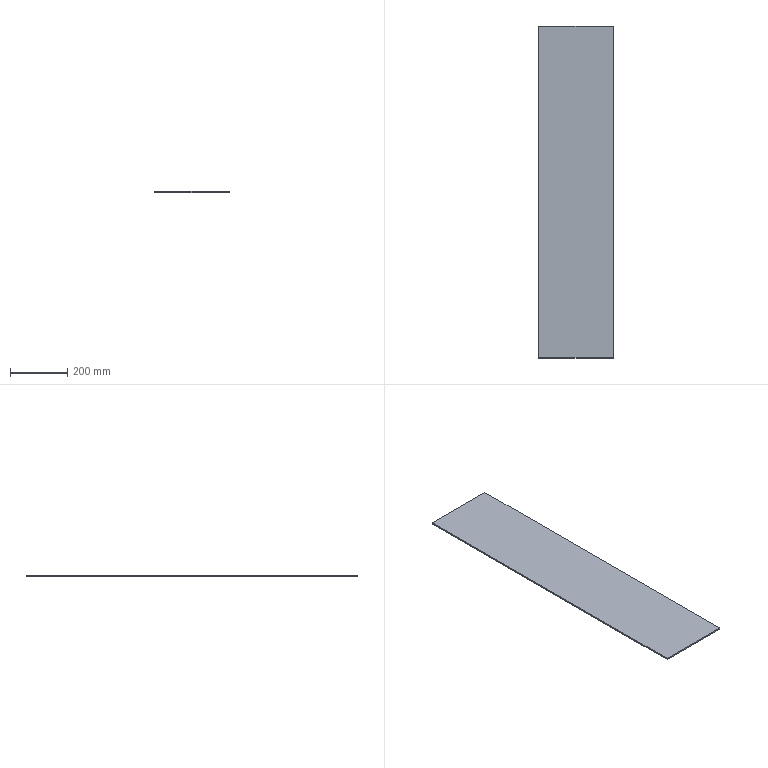Part | SolidWorks | features BaseBody 1 | 1 solid | 6 faces | box 260 x 1160 x 5 mm | volume 1508000 mm3 | plane 6
STEP:
#1=CARTESIAN_POINT('',(-860.,1800.,-395.));
#2=VERTEX_POINT('',#1);
#3=CARTESIAN_POINT('',(-600.,1800.,-395.));
#4=VERTEX_POINT('',#3);
#5=CARTESIAN_POINT('',(-860.,1800.,-395.));
#6=DIRECTION('',(1.,0.,0.));
#7=VECTOR('',#6,1000.);
#8=LINE('',#5,#7);
#9=EDGE_CURVE('',#2,#4,#8,.T.);
#10=ORIENTED_EDGE('',*,*,#9,.F.);
#11=CARTESIAN_POINT('',(-860.,640.,-395.));
#12=VERTEX_POINT('',#11);
#13=CARTESIAN_POINT('',(-860.,640.,-395.));
#14=DIRECTION('',(0.,1.,0.));
#15=VECTOR('',#14,1000.);
#16=LINE('',#13,#15);
#17=EDGE_CURVE('',#12,#2,#16,.T.);
#18=ORIENTED_EDGE('',*,*,#17,.F.);
#19=CARTESIAN_POINT('',(-600.,640.,-395.));
#20=VERTEX_POINT('',#19);
#21=CARTESIAN_POINT('',(-600.,640.,-395.));
#22=DIRECTION('',(-1.,0.,0.));
#23=VECTOR('',#22,1000.);
#24=LINE('',#21,#23);
#25=EDGE_CURVE('',#20,#12,#24,.T.);
#26=ORIENTED_EDGE('',*,*,#25,.F.);
#27=CARTESIAN_POINT('',(-600.,1800.,-395.));
#28=DIRECTION('',(0.,-1.,0.));
#29=VECTOR('',#28,1000.);
#30=LINE('',#27,#29);
#31=EDGE_CURVE('',#4,#20,#30,.T.);
#32=ORIENTED_EDGE('',*,*,#31,.F.);
#33=EDGE_LOOP('',(#10,#18,#26,#32));
#34=FACE_OUTER_BOUND('',#33,.T.);
#35=CARTESIAN_POINT('',(-730.,1220.,-395.));
#36=DIRECTION('',(0.,0.,1.));
#37=DIRECTION('',(1.,0.,0.));
#38=AXIS2_PLACEMENT_3D('',#35,#36,#37);
#39=PLANE('',#38);
#40=ADVANCED_FACE('',(#34),#39,.T.);
#41=CARTESIAN_POINT('',(-600.,1800.,-400.));
#42=VERTEX_POINT('',#41);
#43=CARTESIAN_POINT('',(-860.,1800.,-400.));
#44=VERTEX_POINT('',#43);
#45=CARTESIAN_POINT('',(-600.,1800.,-400.));
#46=DIRECTION('',(-1.,0.,0.));
#47=VECTOR('',#46,1000.);
#48=LINE('',#45,#47);
#49=EDGE_CURVE('',#42,#44,#48,.T.);
#50=ORIENTED_EDGE('',*,*,#49,.F.);
#51=CARTESIAN_POINT('',(-600.,640.,-400.));
#52=VERTEX_POINT('',#51);
#53=CARTESIAN_POINT('',(-600.,640.,-400.));
#54=DIRECTION('',(0.,1.,0.));
#55=VECTOR('',#54,1000.);
#56=LINE('',#53,#55);
#57=EDGE_CURVE('',#52,#42,#56,.T.);
#58=ORIENTED_EDGE('',*,*,#57,.F.);
#59=CARTESIAN_POINT('',(-860.,640.,-400.));
#60=VERTEX_POINT('',#59);
#61=CARTESIAN_POINT('',(-860.,640.,-400.));
#62=DIRECTION('',(1.,0.,0.));
#63=VECTOR('',#62,1000.);
#64=LINE('',#61,#63);
#65=EDGE_CURVE('',#60,#52,#64,.T.);
#66=ORIENTED_EDGE('',*,*,#65,.F.);
#67=CARTESIAN_POINT('',(-860.,1800.,-400.));
#68=DIRECTION('',(0.,-1.,0.));
#69=VECTOR('',#68,1000.);
#70=LINE('',#67,#69);
#71=EDGE_CURVE('',#44,#60,#70,.T.);
#72=ORIENTED_EDGE('',*,*,#71,.F.);
#73=EDGE_LOOP('',(#50,#58,#66,#72));
#74=FACE_OUTER_BOUND('',#73,.T.);
#75=CARTESIAN_POINT('',(-730.,1220.,-400.));
#76=DIRECTION('',(0.,0.,-1.));
#77=DIRECTION('',(0.,-1.,0.));
#78=AXIS2_PLACEMENT_3D('',#75,#76,#77);
#79=PLANE('',#78);
#80=ADVANCED_FACE('',(#74),#79,.T.);
#81=ORIENTED_EDGE('',*,*,#49,.T.);
#82=CARTESIAN_POINT('',(-860.,1800.,-395.));
#83=DIRECTION('',(0.,0.,-1.));
#84=VECTOR('',#83,1000.);
#85=LINE('',#82,#84);
#86=EDGE_CURVE('',#2,#44,#85,.T.);
#87=ORIENTED_EDGE('',*,*,#86,.F.);
#88=ORIENTED_EDGE('',*,*,#9,.T.);
#89=CARTESIAN_POINT('',(-600.,1800.,-400.));
#90=DIRECTION('',(0.,0.,1.));
#91=VECTOR('',#90,1000.);
#92=LINE('',#89,#91);
#93=EDGE_CURVE('',#42,#4,#92,.T.);
#94=ORIENTED_EDGE('',*,*,#93,.F.);
#95=EDGE_LOOP('',(#81,#87,#88,#94));
#96=FACE_OUTER_BOUND('',#95,.T.);
#97=CARTESIAN_POINT('',(-600.,1800.,-400.));
#98=DIRECTION('',(0.,1.,0.));
#99=DIRECTION('',(1.,0.,0.));
#100=AXIS2_PLACEMENT_3D('',#97,#98,#99);
#101=PLANE('',#100);
#102=ADVANCED_FACE('',(#96),#101,.T.);
#103=ORIENTED_EDGE('',*,*,#71,.T.);
#104=CARTESIAN_POINT('',(-860.,640.,-395.));
#105=DIRECTION('',(0.,0.,-1.));
#106=VECTOR('',#105,1000.);
#107=LINE('',#104,#106);
#108=EDGE_CURVE('',#12,#60,#107,.T.);
#109=ORIENTED_EDGE('',*,*,#108,.F.);
#110=ORIENTED_EDGE('',*,*,#17,.T.);
#111=ORIENTED_EDGE('',*,*,#86,.T.);
#112=EDGE_LOOP('',(#103,#109,#110,#111));
#113=FACE_OUTER_BOUND('',#112,.T.);
#114=CARTESIAN_POINT('',(-860.,1800.,-400.));
#115=DIRECTION('',(-1.,0.,0.));
#116=DIRECTION('',(0.,0.,1.));
#117=AXIS2_PLACEMENT_3D('',#114,#115,#116);
#118=PLANE('',#117);
#119=ADVANCED_FACE('',(#113),#118,.T.);
#120=ORIENTED_EDGE('',*,*,#65,.T.);
#121=CARTESIAN_POINT('',(-600.,640.,-395.));
#122=DIRECTION('',(0.,0.,-1.));
#123=VECTOR('',#122,1000.);
#124=LINE('',#121,#123);
#125=EDGE_CURVE('',#20,#52,#124,.T.);
#126=ORIENTED_EDGE('',*,*,#125,.F.);
#127=ORIENTED_EDGE('',*,*,#25,.T.);
#128=ORIENTED_EDGE('',*,*,#108,.T.);
#129=EDGE_LOOP('',(#120,#126,#127,#128));
#130=FACE_OUTER_BOUND('',#129,.T.);
#131=CARTESIAN_POINT('',(-860.,640.,-400.));
#132=DIRECTION('',(0.,-1.,0.));
#133=DIRECTION('',(0.,0.,-1.));
#134=AXIS2_PLACEMENT_3D('',#131,#132,#133);
#135=PLANE('',#134);
#136=ADVANCED_FACE('',(#130),#135,.T.);
#137=ORIENTED_EDGE('',*,*,#57,.T.);
#138=ORIENTED_EDGE('',*,*,#93,.T.);
#139=ORIENTED_EDGE('',*,*,#31,.T.);
#140=ORIENTED_EDGE('',*,*,#125,.T.);
#141=EDGE_LOOP('',(#137,#138,#139,#140));
#142=FACE_OUTER_BOUND('',#141,.T.);
#143=CARTESIAN_POINT('',(-600.,640.,-400.));
#144=DIRECTION('',(1.,0.,0.));
#145=DIRECTION('',(0.,1.,0.));
#146=AXIS2_PLACEMENT_3D('',#143,#144,#145);
#147=PLANE('',#146);
#148=ADVANCED_FACE('',(#142),#147,.T.);
#149=CLOSED_SHELL('',(#40,#80,#102,#119,#136,#148));
#150=MANIFOLD_SOLID_BREP('',#149);
#151=CARTESIAN_POINT('',(0.,0.,0.));
#152=DIRECTION('',(0.,0.,1.));
#153=DIRECTION('',(1.,0.,0.));
#154=AXIS2_PLACEMENT_3D('',#151,#152,#153);
#155=(LENGTH_UNIT()NAMED_UNIT(*)SI_UNIT(.MILLI.,.METRE.));
#156=UNCERTAINTY_MEASURE_WITH_UNIT(LENGTH_MEASURE(0.00001),#155,'','');
#157=(NAMED_UNIT(*)PLANE_ANGLE_UNIT()SI_UNIT($,.RADIAN.));
#158=(NAMED_UNIT(*)SI_UNIT($,.STERADIAN.)SOLID_ANGLE_UNIT());
#159=(GEOMETRIC_REPRESENTATION_CONTEXT(3)GLOBAL_UNCERTAINTY_ASSIGNED_CONTEXT((#156))GLOBAL_UNIT_ASSIGNED_CONTEXT((#155,#157,#158))REPRESENTATION_CONTEXT('',''));
#160=ADVANCED_BREP_SHAPE_REPRESENTATION('',(#150,#154),#159);